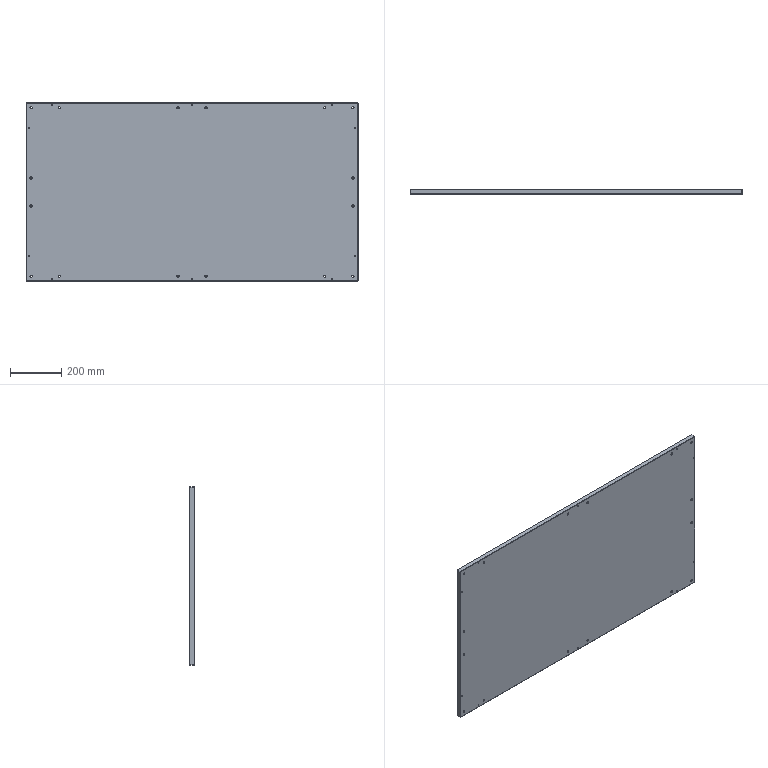Part | SolidWorks | features MirrorPattern 5, 3DProfileFeature 4, HoleWzd 4, LPattern 4, Chamfer 1, Extrusion 1 | 1 solid | 126 faces | box 1300 x 20 x 700 mm | volume 18144468 mm3 | cylinder 84 | plane 42 | commonest cylinder face diameters 9 x32 15 x32 4.2 x20